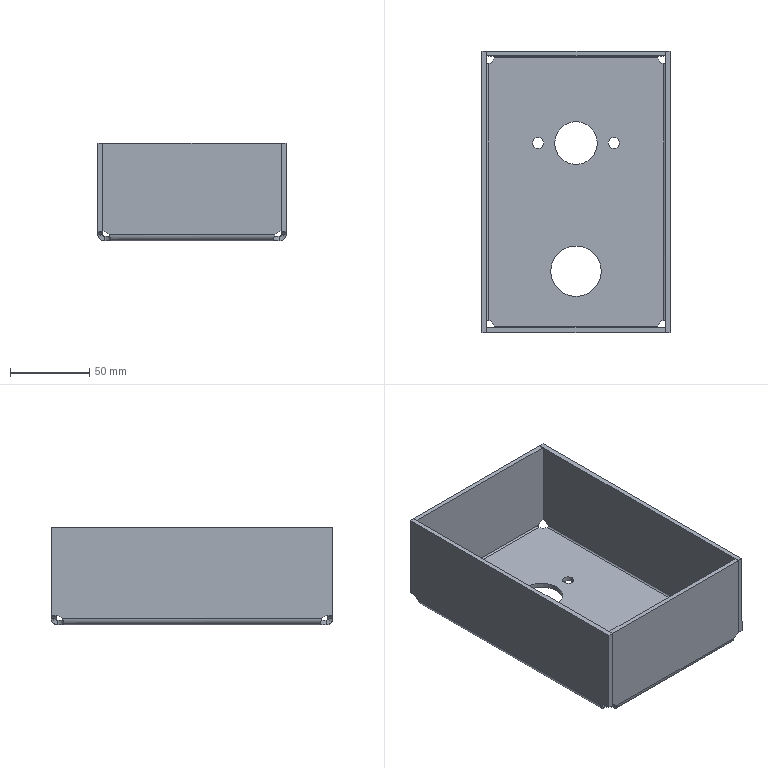Part | SolidWorks | features Extrusion 1, FlatPattern 1, SM3dBend 1, SheetMetal 1, SolidToSheetMetal 1 | 1 solid | 62 faces | box 119 x 178 x 61.873 mm | volume 159219 mm3 | cylinder 28 | plane 26 | spline 8 | commonest cylinder face diameters 10 x12 2 x4 7 x4 8 x4 27 x2 32 x2